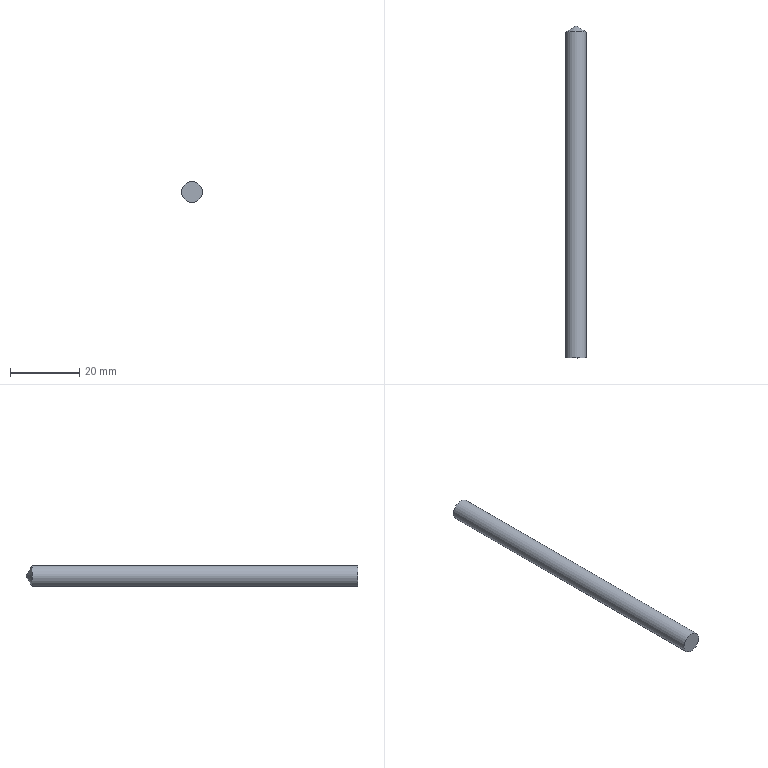Part | NX | features solid 2 | 1 solid | 3 faces | box 6 x 95.732 x 6 mm | volume 2674 mm3 | cylinder 1 | plane 1 | cone 1 | commonest cylinder face diameters 6 x1
STEP:
#1=CARTESIAN_POINT('',(-88.,-26.,55.));
#2=VERTEX_POINT('',#1);
#3=CARTESIAN_POINT('',(-85.,-26.,55.));
#4=DIRECTION('',(0.,1.,0.));
#5=DIRECTION('',(-1.,0.,0.));
#6=AXIS2_PLACEMENT_3D('',#3,#4,#5);
#7=CIRCLE('',#6,3.);
#8=EDGE_CURVE('',#2,#2,#7,.T.);
#9=ORIENTED_EDGE('',*,*,#8,.F.);
#10=EDGE_LOOP('',(#9));
#11=FACE_BOUND('',#10,.T.);
#12=CARTESIAN_POINT('',(-88.,-120.,55.));
#13=VERTEX_POINT('',#12);
#14=CARTESIAN_POINT('',(-85.,-120.,55.));
#15=DIRECTION('',(0.,1.,0.));
#16=DIRECTION('',(-1.,0.,0.));
#17=AXIS2_PLACEMENT_3D('',#14,#15,#16);
#18=CIRCLE('',#17,3.);
#19=EDGE_CURVE('',#13,#13,#18,.T.);
#20=ORIENTED_EDGE('',*,*,#19,.T.);
#21=EDGE_LOOP('',(#20));
#22=FACE_BOUND('',#21,.T.);
#23=CARTESIAN_POINT('',(-85.,-30.,55.));
#24=DIRECTION('',(0.,-1.,0.));
#25=DIRECTION('',(1.,0.,0.));
#26=AXIS2_PLACEMENT_3D('',#23,#24,#25);
#27=CYLINDRICAL_SURFACE('',#26,3.);
#28=ADVANCED_FACE('',(#11,#22),#27,.T.);
#29=ORIENTED_EDGE('',*,*,#19,.F.);
#30=EDGE_LOOP('',(#29));
#31=FACE_BOUND('',#30,.T.);
#32=CARTESIAN_POINT('',(-85.,-120.,55.));
#33=DIRECTION('',(0.,1.,0.));
#34=DIRECTION('',(-1.,0.,0.));
#35=AXIS2_PLACEMENT_3D('',#32,#33,#34);
#36=PLANE('',#35);
#37=ADVANCED_FACE('',(#31),#36,.F.);
#38=ORIENTED_EDGE('',*,*,#8,.T.);
#39=EDGE_LOOP('',(#38));
#40=FACE_BOUND('',#39,.T.);
#41=CARTESIAN_POINT('',(-85.,-24.268,55.));
#42=VERTEX_POINT('',#41);
#43=VERTEX_LOOP('',#42);
#44=FACE_BOUND('',#43,.T.);
#45=CARTESIAN_POINT('',(-85.,-24.268,55.));
#46=DIRECTION('',(0.,-1.,0.));
#47=DIRECTION('',(1.,0.,0.));
#48=AXIS2_PLACEMENT_3D('',#45,#46,#47);
#49=CONICAL_SURFACE('',#48,0.,1.047);
#50=ADVANCED_FACE('',(#40,#44),#49,.T.);
#51=CLOSED_SHELL('',(#28,#37,#50));
#52=MANIFOLD_SOLID_BREP('',#51);
#53=(LENGTH_UNIT()NAMED_UNIT(*)SI_UNIT(.MILLI.,.METRE.));
#54=UNCERTAINTY_MEASURE_WITH_UNIT(LENGTH_MEASURE(0.00001),#53,'','');
#55=(NAMED_UNIT(*)PLANE_ANGLE_UNIT()SI_UNIT($,.RADIAN.));
#56=(NAMED_UNIT(*)SI_UNIT($,.STERADIAN.)SOLID_ANGLE_UNIT());
#57=(GEOMETRIC_REPRESENTATION_CONTEXT(3)GLOBAL_UNCERTAINTY_ASSIGNED_CONTEXT((#54))GLOBAL_UNIT_ASSIGNED_CONTEXT((#53,#55,#56))REPRESENTATION_CONTEXT('',''));
#58=ADVANCED_BREP_SHAPE_REPRESENTATION('',(#52),#57);